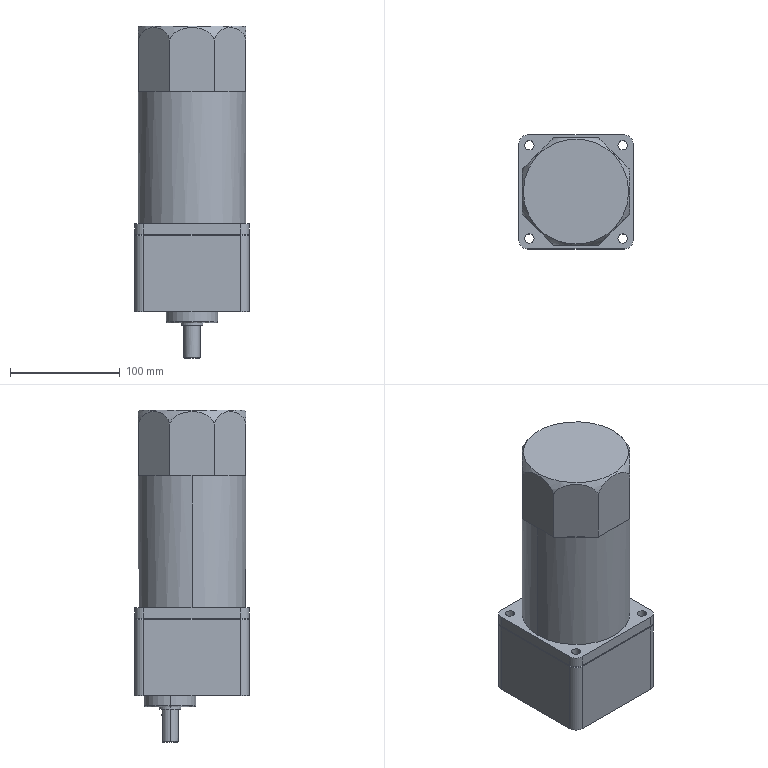Part | STEP file | DDK250W50 electromagnetic brake motor | 1 solid | 83 faces | box 104 x 104 x 302.5 mm | volume 2241190 mm3 | plane 42 | cylinder 27 | cone 10 | spline 4 | commonest cylinder face diameters 8.5 x8 16 x8 15 x2 20 x2 47 x2 94 x2